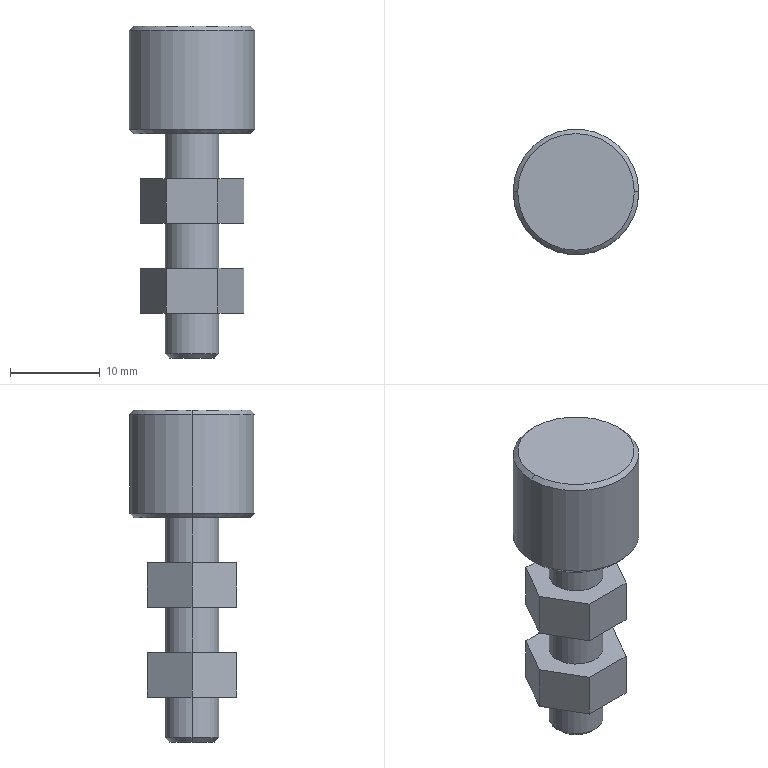Part | STEP file | aluminium profile door-catch magnet post | 1 solid | 33 faces | box 14 x 14 x 37 mm | volume 3124 mm3 | plane 19 | cylinder 8 | cone 6 | commonest cylinder face diameters 6 x6 14 x2